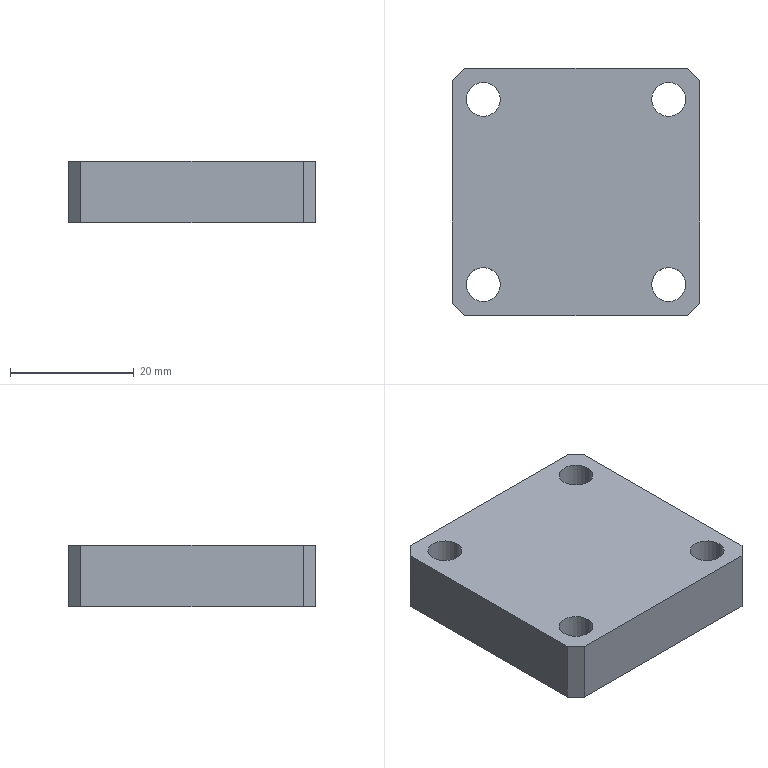Part | SolidWorks | features BaseBody 1 | 1 solid | 30 faces | box 40 x 40 x 10 mm | volume 13952 mm3 | cylinder 16 | plane 14 | commonest cylinder face diameters 5.5 x8 9.5 x8
STEP:
#1=CARTESIAN_POINT('',(19.75,15.,5.4));
#2=VERTEX_POINT('',#1);
#3=CARTESIAN_POINT('',(10.25,15.,5.4));
#4=VERTEX_POINT('',#3);
#5=CARTESIAN_POINT('',(15.,15.,5.4));
#6=DIRECTION('',(0.,0.,-1.));
#7=DIRECTION('',(-1.,0.,0.));
#8=AXIS2_PLACEMENT_3D('',#5,#6,#7);
#9=CIRCLE('',#8,4.75);
#10=EDGE_CURVE('',#2,#4,#9,.T.);
#11=ORIENTED_EDGE('',*,*,#10,.F.);
#12=CARTESIAN_POINT('',(19.75,15.,0.));
#13=VERTEX_POINT('',#12);
#14=CARTESIAN_POINT('',(19.75,15.,0.));
#15=DIRECTION('',(0.,0.,-1.));
#16=VECTOR('',#15,1000.);
#17=LINE('',#14,#16);
#18=EDGE_CURVE('',#2,#13,#17,.T.);
#19=ORIENTED_EDGE('',*,*,#18,.T.);
#20=CARTESIAN_POINT('',(10.25,15.,0.));
#21=VERTEX_POINT('',#20);
#22=CARTESIAN_POINT('',(15.,15.,0.));
#23=DIRECTION('',(0.,0.,-1.));
#24=DIRECTION('',(-1.,0.,0.));
#25=AXIS2_PLACEMENT_3D('',#22,#23,#24);
#26=CIRCLE('',#25,4.75);
#27=EDGE_CURVE('',#13,#21,#26,.T.);
#28=ORIENTED_EDGE('',*,*,#27,.T.);
#29=CARTESIAN_POINT('',(10.25,15.,0.));
#30=DIRECTION('',(0.,0.,-1.));
#31=VECTOR('',#30,1000.);
#32=LINE('',#29,#31);
#33=EDGE_CURVE('',#4,#21,#32,.T.);
#34=ORIENTED_EDGE('',*,*,#33,.F.);
#35=EDGE_LOOP('',(#11,#19,#28,#34));
#36=FACE_OUTER_BOUND('',#35,.T.);
#37=CARTESIAN_POINT('',(15.,15.,0.));
#38=DIRECTION('',(0.,0.,-1.));
#39=DIRECTION('',(-1.,0.,0.));
#40=AXIS2_PLACEMENT_3D('',#37,#38,#39);
#41=CYLINDRICAL_SURFACE('',#40,4.75);
#42=ADVANCED_FACE('',(#36),#41,.F.);
#43=CARTESIAN_POINT('',(17.75,15.,10.));
#44=VERTEX_POINT('',#43);
#45=CARTESIAN_POINT('',(12.25,15.,10.));
#46=VERTEX_POINT('',#45);
#47=CARTESIAN_POINT('',(15.,15.,10.));
#48=DIRECTION('',(0.,0.,-1.));
#49=DIRECTION('',(-1.,0.,0.));
#50=AXIS2_PLACEMENT_3D('',#47,#48,#49);
#51=CIRCLE('',#50,2.75);
#52=EDGE_CURVE('',#44,#46,#51,.T.);
#53=ORIENTED_EDGE('',*,*,#52,.F.);
#54=CARTESIAN_POINT('',(17.75,15.,5.4));
#55=VERTEX_POINT('',#54);
#56=CARTESIAN_POINT('',(17.75,15.,0.));
#57=DIRECTION('',(0.,0.,-1.));
#58=VECTOR('',#57,1000.);
#59=LINE('',#56,#58);
#60=EDGE_CURVE('',#44,#55,#59,.T.);
#61=ORIENTED_EDGE('',*,*,#60,.T.);
#62=CARTESIAN_POINT('',(12.25,15.,5.4));
#63=VERTEX_POINT('',#62);
#64=CARTESIAN_POINT('',(15.,15.,5.4));
#65=DIRECTION('',(0.,0.,-1.));
#66=DIRECTION('',(-1.,0.,0.));
#67=AXIS2_PLACEMENT_3D('',#64,#65,#66);
#68=CIRCLE('',#67,2.75);
#69=EDGE_CURVE('',#55,#63,#68,.T.);
#70=ORIENTED_EDGE('',*,*,#69,.T.);
#71=CARTESIAN_POINT('',(12.25,15.,0.));
#72=DIRECTION('',(0.,0.,-1.));
#73=VECTOR('',#72,1000.);
#74=LINE('',#71,#73);
#75=EDGE_CURVE('',#46,#63,#74,.T.);
#76=ORIENTED_EDGE('',*,*,#75,.F.);
#77=EDGE_LOOP('',(#53,#61,#70,#76));
#78=FACE_OUTER_BOUND('',#77,.T.);
#79=CARTESIAN_POINT('',(15.,15.,0.));
#80=DIRECTION('',(0.,0.,-1.));
#81=DIRECTION('',(-1.,0.,0.));
#82=AXIS2_PLACEMENT_3D('',#79,#80,#81);
#83=CYLINDRICAL_SURFACE('',#82,2.75);
#84=ADVANCED_FACE('',(#78),#83,.F.);
#85=CARTESIAN_POINT('',(-10.25,15.,5.4));
#86=VERTEX_POINT('',#85);
#87=CARTESIAN_POINT('',(-19.75,15.,5.4));
#88=VERTEX_POINT('',#87);
#89=CARTESIAN_POINT('',(-15.,15.,5.4));
#90=DIRECTION('',(0.,0.,-1.));
#91=DIRECTION('',(-1.,0.,0.));
#92=AXIS2_PLACEMENT_3D('',#89,#90,#91);
#93=CIRCLE('',#92,4.75);
#94=EDGE_CURVE('',#86,#88,#93,.T.);
#95=ORIENTED_EDGE('',*,*,#94,.F.);
#96=CARTESIAN_POINT('',(-10.25,15.,0.));
#97=VERTEX_POINT('',#96);
#98=CARTESIAN_POINT('',(-10.25,15.,0.));
#99=DIRECTION('',(0.,0.,-1.));
#100=VECTOR('',#99,1000.);
#101=LINE('',#98,#100);
#102=EDGE_CURVE('',#86,#97,#101,.T.);
#103=ORIENTED_EDGE('',*,*,#102,.T.);
#104=CARTESIAN_POINT('',(-19.75,15.,0.));
#105=VERTEX_POINT('',#104);
#106=CARTESIAN_POINT('',(-15.,15.,0.));
#107=DIRECTION('',(0.,0.,-1.));
#108=DIRECTION('',(-1.,0.,0.));
#109=AXIS2_PLACEMENT_3D('',#106,#107,#108);
#110=CIRCLE('',#109,4.75);
#111=EDGE_CURVE('',#97,#105,#110,.T.);
#112=ORIENTED_EDGE('',*,*,#111,.T.);
#113=CARTESIAN_POINT('',(-19.75,15.,0.));
#114=DIRECTION('',(0.,0.,-1.));
#115=VECTOR('',#114,1000.);
#116=LINE('',#113,#115);
#117=EDGE_CURVE('',#88,#105,#116,.T.);
#118=ORIENTED_EDGE('',*,*,#117,.F.);
#119=EDGE_LOOP('',(#95,#103,#112,#118));
#120=FACE_OUTER_BOUND('',#119,.T.);
#121=CARTESIAN_POINT('',(-15.,15.,0.));
#122=DIRECTION('',(0.,0.,-1.));
#123=DIRECTION('',(-1.,0.,0.));
#124=AXIS2_PLACEMENT_3D('',#121,#122,#123);
#125=CYLINDRICAL_SURFACE('',#124,4.75);
#126=ADVANCED_FACE('',(#120),#125,.F.);
#127=CARTESIAN_POINT('',(-12.25,15.,10.));
#128=VERTEX_POINT('',#127);
#129=CARTESIAN_POINT('',(-17.75,15.,10.));
#130=VERTEX_POINT('',#129);
#131=CARTESIAN_POINT('',(-15.,15.,10.));
#132=DIRECTION('',(0.,0.,-1.));
#133=DIRECTION('',(-1.,0.,0.));
#134=AXIS2_PLACEMENT_3D('',#131,#132,#133);
#135=CIRCLE('',#134,2.75);
#136=EDGE_CURVE('',#128,#130,#135,.T.);
#137=ORIENTED_EDGE('',*,*,#136,.F.);
#138=CARTESIAN_POINT('',(-12.25,15.,5.4));
#139=VERTEX_POINT('',#138);
#140=CARTESIAN_POINT('',(-12.25,15.,0.));
#141=DIRECTION('',(0.,0.,-1.));
#142=VECTOR('',#141,1000.);
#143=LINE('',#140,#142);
#144=EDGE_CURVE('',#128,#139,#143,.T.);
#145=ORIENTED_EDGE('',*,*,#144,.T.);
#146=CARTESIAN_POINT('',(-17.75,15.,5.4));
#147=VERTEX_POINT('',#146);
#148=CARTESIAN_POINT('',(-15.,15.,5.4));
#149=DIRECTION('',(0.,0.,-1.));
#150=DIRECTION('',(-1.,0.,0.));
#151=AXIS2_PLACEMENT_3D('',#148,#149,#150);
#152=CIRCLE('',#151,2.75);
#153=EDGE_CURVE('',#139,#147,#152,.T.);
#154=ORIENTED_EDGE('',*,*,#153,.T.);
#155=CARTESIAN_POINT('',(-17.75,15.,0.));
#156=DIRECTION('',(0.,0.,-1.));
#157=VECTOR('',#156,1000.);
#158=LINE('',#155,#157);
#159=EDGE_CURVE('',#130,#147,#158,.T.);
#160=ORIENTED_EDGE('',*,*,#159,.F.);
#161=EDGE_LOOP('',(#137,#145,#154,#160));
#162=FACE_OUTER_BOUND('',#161,.T.);
#163=CARTESIAN_POINT('',(-15.,15.,0.));
#164=DIRECTION('',(0.,0.,-1.));
#165=DIRECTION('',(-1.,0.,0.));
#166=AXIS2_PLACEMENT_3D('',#163,#164,#165);
#167=CYLINDRICAL_SURFACE('',#166,2.75);
#168=ADVANCED_FACE('',(#162),#167,.F.);
#169=CARTESIAN_POINT('',(19.75,-15.,5.4));
#170=VERTEX_POINT('',#169);
#171=CARTESIAN_POINT('',(10.25,-15.,5.4));
#172=VERTEX_POINT('',#171);
#173=CARTESIAN_POINT('',(15.,-15.,5.4));
#174=DIRECTION('',(0.,0.,-1.));
#175=DIRECTION('',(-1.,0.,0.));
#176=AXIS2_PLACEMENT_3D('',#173,#174,#175);
#177=CIRCLE('',#176,4.75);
#178=EDGE_CURVE('',#170,#172,#177,.T.);
#179=ORIENTED_EDGE('',*,*,#178,.F.);
#180=CARTESIAN_POINT('',(19.75,-15.,0.));
#181=VERTEX_POINT('',#180);
#182=CARTESIAN_POINT('',(19.75,-15.,0.));
#183=DIRECTION('',(0.,0.,-1.));
#184=VECTOR('',#183,1000.);
#185=LINE('',#182,#184);
#186=EDGE_CURVE('',#170,#181,#185,.T.);
#187=ORIENTED_EDGE('',*,*,#186,.T.);
#188=CARTESIAN_POINT('',(10.25,-15.,0.));
#189=VERTEX_POINT('',#188);
#190=CARTESIAN_POINT('',(15.,-15.,0.));
#191=DIRECTION('',(0.,0.,-1.));
#192=DIRECTION('',(-1.,0.,0.));
#193=AXIS2_PLACEMENT_3D('',#190,#191,#192);
#194=CIRCLE('',#193,4.75);
#195=EDGE_CURVE('',#181,#189,#194,.T.);
#196=ORIENTED_EDGE('',*,*,#195,.T.);
#197=CARTESIAN_POINT('',(10.25,-15.,0.));
#198=DIRECTION('',(0.,0.,-1.));
#199=VECTOR('',#198,1000.);
#200=LINE('',#197,#199);
#201=EDGE_CURVE('',#172,#189,#200,.T.);
#202=ORIENTED_EDGE('',*,*,#201,.F.);
#203=EDGE_LOOP('',(#179,#187,#196,#202));
#204=FACE_OUTER_BOUND('',#203,.T.);
#205=CARTESIAN_POINT('',(15.,-15.,0.));
#206=DIRECTION('',(0.,0.,-1.));
#207=DIRECTION('',(-1.,0.,0.));
#208=AXIS2_PLACEMENT_3D('',#205,#206,#207);
#209=CYLINDRICAL_SURFACE('',#208,4.75);
#210=ADVANCED_FACE('',(#204),#209,.F.);
#211=CARTESIAN_POINT('',(17.75,-15.,10.));
#212=VERTEX_POINT('',#211);
#213=CARTESIAN_POINT('',(12.25,-15.,10.));
#214=VERTEX_POINT('',#213);
#215=CARTESIAN_POINT('',(15.,-15.,10.));
#216=DIRECTION('',(0.,0.,-1.));
#217=DIRECTION('',(-1.,0.,0.));
#218=AXIS2_PLACEMENT_3D('',#215,#216,#217);
#219=CIRCLE('',#218,2.75);
#220=EDGE_CURVE('',#212,#214,#219,.T.);
#221=ORIENTED_EDGE('',*,*,#220,.F.);
#222=CARTESIAN_POINT('',(17.75,-15.,5.4));
#223=VERTEX_POINT('',#222);
#224=CARTESIAN_POINT('',(17.75,-15.,0.));
#225=DIRECTION('',(0.,0.,-1.));
#226=VECTOR('',#225,1000.);
#227=LINE('',#224,#226);
#228=EDGE_CURVE('',#212,#223,#227,.T.);
#229=ORIENTED_EDGE('',*,*,#228,.T.);
#230=CARTESIAN_POINT('',(12.25,-15.,5.4));
#231=VERTEX_POINT('',#230);
#232=CARTESIAN_POINT('',(15.,-15.,5.4));
#233=DIRECTION('',(0.,0.,-1.));
#234=DIRECTION('',(-1.,0.,0.));
#235=AXIS2_PLACEMENT_3D('',#232,#233,#234);
#236=CIRCLE('',#235,2.75);
#237=EDGE_CURVE('',#223,#231,#236,.T.);
#238=ORIENTED_EDGE('',*,*,#237,.T.);
#239=CARTESIAN_POINT('',(12.25,-15.,0.));
#240=DIRECTION('',(0.,0.,-1.));
#241=VECTOR('',#240,1000.);
#242=LINE('',#239,#241);
#243=EDGE_CURVE('',#214,#231,#242,.T.);
#244=ORIENTED_EDGE('',*,*,#243,.F.);
#245=EDGE_LOOP('',(#221,#229,#238,#244));
#246=FACE_OUTER_BOUND('',#245,.T.);
#247=CARTESIAN_POINT('',(15.,-15.,0.));
#248=DIRECTION('',(0.,0.,-1.));
#249=DIRECTION('',(-1.,0.,0.));
#250=AXIS2_PLACEMENT_3D('',#247,#248,#249);
#251=CYLINDRICAL_SURFACE('',#250,2.75);
#252=ADVANCED_FACE('',(#246),#251,.F.);
#253=CARTESIAN_POINT('',(-10.25,-15.,5.4));
#254=VERTEX_POINT('',#253);
#255=CARTESIAN_POINT('',(-19.75,-15.,5.4));
#256=VERTEX_POINT('',#255);
#257=CARTESIAN_POINT('',(-15.,-15.,5.4));
#258=DIRECTION('',(0.,0.,-1.));
#259=DIRECTION('',(-1.,0.,0.));
#260=AXIS2_PLACEMENT_3D('',#257,#258,#259);
#261=CIRCLE('',#260,4.75);
#262=EDGE_CURVE('',#254,#256,#261,.T.);
#263=ORIENTED_EDGE('',*,*,#262,.F.);
#264=CARTESIAN_POINT('',(-10.25,-15.,0.));
#265=VERTEX_POINT('',#264);
#266=CARTESIAN_POINT('',(-10.25,-15.,0.));
#267=DIRECTION('',(0.,0.,-1.));
#268=VECTOR('',#267,1000.);
#269=LINE('',#266,#268);
#270=EDGE_CURVE('',#254,#265,#269,.T.);
#271=ORIENTED_EDGE('',*,*,#270,.T.);
#272=CARTESIAN_POINT('',(-19.75,-15.,0.));
#273=VERTEX_POINT('',#272);
#274=CARTESIAN_POINT('',(-15.,-15.,0.));
#275=DIRECTION('',(0.,0.,-1.));
#276=DIRECTION('',(-1.,0.,0.));
#277=AXIS2_PLACEMENT_3D('',#274,#275,#276);
#278=CIRCLE('',#277,4.75);
#279=EDGE_CURVE('',#265,#273,#278,.T.);
#280=ORIENTED_EDGE('',*,*,#279,.T.);
#281=CARTESIAN_POINT('',(-19.75,-15.,0.));
#282=DIRECTION('',(0.,0.,-1.));
#283=VECTOR('',#282,1000.);
#284=LINE('',#281,#283);
#285=EDGE_CURVE('',#256,#273,#284,.T.);
#286=ORIENTED_EDGE('',*,*,#285,.F.);
#287=EDGE_LOOP('',(#263,#271,#280,#286));
#288=FACE_OUTER_BOUND('',#287,.T.);
#289=CARTESIAN_POINT('',(-15.,-15.,0.));
#290=DIRECTION('',(0.,0.,-1.));
#291=DIRECTION('',(-1.,0.,0.));
#292=AXIS2_PLACEMENT_3D('',#289,#290,#291);
#293=CYLINDRICAL_SURFACE('',#292,4.75);
#294=ADVANCED_FACE('',(#288),#293,.F.);
#295=CARTESIAN_POINT('',(-12.25,-15.,10.));
#296=VERTEX_POINT('',#295);
#297=CARTESIAN_POINT('',(-17.75,-15.,10.));
#298=VERTEX_POINT('',#297);
#299=CARTESIAN_POINT('',(-15.,-15.,10.));
#300=DIRECTION('',(0.,0.,-1.));
#301=DIRECTION('',(-1.,0.,0.));
#302=AXIS2_PLACEMENT_3D('',#299,#300,#301);
#303=CIRCLE('',#302,2.75);
#304=EDGE_CURVE('',#296,#298,#303,.T.);
#305=ORIENTED_EDGE('',*,*,#304,.F.);
#306=CARTESIAN_POINT('',(-12.25,-15.,5.4));
#307=VERTEX_POINT('',#306);
#308=CARTESIAN_POINT('',(-12.25,-15.,0.));
#309=DIRECTION('',(0.,0.,-1.));
#310=VECTOR('',#309,1000.);
#311=LINE('',#308,#310);
#312=EDGE_CURVE('',#296,#307,#311,.T.);
#313=ORIENTED_EDGE('',*,*,#312,.T.);
#314=CARTESIAN_POINT('',(-17.75,-15.,5.4));
#315=VERTEX_POINT('',#314);
#316=CARTESIAN_POINT('',(-15.,-15.,5.4));
#317=DIRECTION('',(0.,0.,-1.));
#318=DIRECTION('',(-1.,0.,0.));
#319=AXIS2_PLACEMENT_3D('',#316,#317,#318);
#320=CIRCLE('',#319,2.75);
#321=EDGE_CURVE('',#307,#315,#320,.T.);
#322=ORIENTED_EDGE('',*,*,#321,.T.);
#323=CARTESIAN_POINT('',(-17.75,-15.,0.));
#324=DIRECTION('',(0.,0.,-1.));
#325=VECTOR('',#324,1000.);
#326=LINE('',#323,#325);
#327=EDGE_CURVE('',#298,#315,#326,.T.);
#328=ORIENTED_EDGE('',*,*,#327,.F.);
#329=EDGE_LOOP('',(#305,#313,#322,#328));
#330=FACE_OUTER_BOUND('',#329,.T.);
#331=CARTESIAN_POINT('',(-15.,-15.,0.));
#332=DIRECTION('',(0.,0.,-1.));
#333=DIRECTION('',(-1.,0.,0.));
#334=AXIS2_PLACEMENT_3D('',#331,#332,#333);
#335=CYLINDRICAL_SURFACE('',#334,2.75);
#336=ADVANCED_FACE('',(#330),#335,.F.);
#337=CARTESIAN_POINT('',(-20.,18.,0.));
#338=VERTEX_POINT('',#337);
#339=CARTESIAN_POINT('',(-20.,-18.,0.));
#340=VERTEX_POINT('',#339);
#341=CARTESIAN_POINT('',(-20.,20.,0.));
#342=DIRECTION('',(0.,-1.,0.));
#343=VECTOR('',#342,1000.);
#344=LINE('',#341,#343);
#345=EDGE_CURVE('',#338,#340,#344,.T.);
#346=ORIENTED_EDGE('',*,*,#345,.T.);
#347=CARTESIAN_POINT('',(-20.,-18.,10.));
#348=VERTEX_POINT('',#347);
#349=CARTESIAN_POINT('',(-20.,-18.,10.));
#350=DIRECTION('',(0.,0.,1.));
#351=VECTOR('',#350,1000.);
#352=LINE('',#349,#351);
#353=EDGE_CURVE('',#340,#348,#352,.T.);
#354=ORIENTED_EDGE('',*,*,#353,.T.);
#355=CARTESIAN_POINT('',(-20.,18.,10.));
#356=VERTEX_POINT('',#355);
#357=CARTESIAN_POINT('',(-20.,20.,10.));
#358=DIRECTION('',(0.,-1.,0.));
#359=VECTOR('',#358,1000.);
#360=LINE('',#357,#359);
#361=EDGE_CURVE('',#356,#348,#360,.T.);
#362=ORIENTED_EDGE('',*,*,#361,.F.);
#363=CARTESIAN_POINT('',(-20.,18.,10.));
#364=DIRECTION('',(0.,0.,-1.));
#365=VECTOR('',#364,1000.);
#366=LINE('',#363,#365);
#367=EDGE_CURVE('',#356,#338,#366,.T.);
#368=ORIENTED_EDGE('',*,*,#367,.T.);
#369=EDGE_LOOP('',(#346,#354,#362,#368));
#370=FACE_OUTER_BOUND('',#369,.T.);
#371=CARTESIAN_POINT('',(-20.,20.,10.));
#372=DIRECTION('',(1.,0.,0.));
#373=DIRECTION('',(0.,1.,0.));
#374=AXIS2_PLACEMENT_3D('',#371,#372,#373);
#375=PLANE('',#374);
#376=ADVANCED_FACE('',(#370),#375,.F.);
#377=CARTESIAN_POINT('',(-18.,-20.,10.));
#378=VERTEX_POINT('',#377);
#379=CARTESIAN_POINT('',(18.,-20.,10.));
#380=VERTEX_POINT('',#379);
#381=CARTESIAN_POINT('',(20.,-20.,10.));
#382=DIRECTION('',(1.,0.,0.));
#383=VECTOR('',#382,1000.);
#384=LINE('',#381,#383);
#385=EDGE_CURVE('',#378,#380,#384,.T.);
#386=ORIENTED_EDGE('',*,*,#385,.F.);
#387=CARTESIAN_POINT('',(-18.,-20.,0.));
#388=VERTEX_POINT('',#387);
#389=CARTESIAN_POINT('',(-18.,-20.,10.));
#390=DIRECTION('',(0.,0.,-1.));
#391=VECTOR('',#390,1000.);
#392=LINE('',#389,#391);
#393=EDGE_CURVE('',#378,#388,#392,.T.);
#394=ORIENTED_EDGE('',*,*,#393,.T.);
#395=CARTESIAN_POINT('',(18.,-20.,0.));
#396=VERTEX_POINT('',#395);
#397=CARTESIAN_POINT('',(20.,-20.,0.));
#398=DIRECTION('',(1.,0.,0.));
#399=VECTOR('',#398,1000.);
#400=LINE('',#397,#399);
#401=EDGE_CURVE('',#388,#396,#400,.T.);
#402=ORIENTED_EDGE('',*,*,#401,.T.);
#403=CARTESIAN_POINT('',(18.,-20.,10.));
#404=DIRECTION('',(0.,0.,1.));
#405=VECTOR('',#404,1000.);
#406=LINE('',#403,#405);
#407=EDGE_CURVE('',#396,#380,#406,.T.);
#408=ORIENTED_EDGE('',*,*,#407,.T.);
#409=EDGE_LOOP('',(#386,#394,#402,#408));
#410=FACE_OUTER_BOUND('',#409,.T.);
#411=CARTESIAN_POINT('',(20.,-20.,10.));
#412=DIRECTION('',(0.,1.,0.));
#413=DIRECTION('',(-1.,0.,0.));
#414=AXIS2_PLACEMENT_3D('',#411,#412,#413);
#415=PLANE('',#414);
#416=ADVANCED_FACE('',(#410),#415,.F.);
#417=CARTESIAN_POINT('',(20.,-18.,10.));
#418=VERTEX_POINT('',#417);
#419=CARTESIAN_POINT('',(20.,18.,10.));
#420=VERTEX_POINT('',#419);
#421=CARTESIAN_POINT('',(20.,20.,10.));
#422=DIRECTION('',(0.,1.,0.));
#423=VECTOR('',#422,1000.);
#424=LINE('',#421,#423);
#425=EDGE_CURVE('',#418,#420,#424,.T.);
#426=ORIENTED_EDGE('',*,*,#425,.F.);
#427=CARTESIAN_POINT('',(20.,-18.,0.));
#428=VERTEX_POINT('',#427);
#429=CARTESIAN_POINT('',(20.,-18.,10.));
#430=DIRECTION('',(0.,0.,-1.));
#431=VECTOR('',#430,1000.);
#432=LINE('',#429,#431);
#433=EDGE_CURVE('',#418,#428,#432,.T.);
#434=ORIENTED_EDGE('',*,*,#433,.T.);
#435=CARTESIAN_POINT('',(20.,18.,0.));
#436=VERTEX_POINT('',#435);
#437=CARTESIAN_POINT('',(20.,20.,0.));
#438=DIRECTION('',(0.,1.,0.));
#439=VECTOR('',#438,1000.);
#440=LINE('',#437,#439);
#441=EDGE_CURVE('',#428,#436,#440,.T.);
#442=ORIENTED_EDGE('',*,*,#441,.T.);
#443=CARTESIAN_POINT('',(20.,18.,10.));
#444=DIRECTION('',(0.,0.,1.));
#445=VECTOR('',#444,1000.);
#446=LINE('',#443,#445);
#447=EDGE_CURVE('',#436,#420,#446,.T.);
#448=ORIENTED_EDGE('',*,*,#447,.T.);
#449=EDGE_LOOP('',(#426,#434,#442,#448));
#450=FACE_OUTER_BOUND('',#449,.T.);
#451=CARTESIAN_POINT('',(20.,20.,10.));
#452=DIRECTION('',(-1.,0.,0.));
#453=DIRECTION('',(0.,-1.,0.));
#454=AXIS2_PLACEMENT_3D('',#451,#452,#453);
#455=PLANE('',#454);
#456=ADVANCED_FACE('',(#450),#455,.F.);
#457=CARTESIAN_POINT('',(18.,20.,0.));
#458=VERTEX_POINT('',#457);
#459=CARTESIAN_POINT('',(-18.,20.,0.));
#460=VERTEX_POINT('',#459);
#461=CARTESIAN_POINT('',(20.,20.,0.));
#462=DIRECTION('',(-1.,0.,0.));
#463=VECTOR('',#462,1000.);
#464=LINE('',#461,#463);
#465=EDGE_CURVE('',#458,#460,#464,.T.);
#466=ORIENTED_EDGE('',*,*,#465,.T.);
#467=CARTESIAN_POINT('',(-18.,20.,10.));
#468=VERTEX_POINT('',#467);
#469=CARTESIAN_POINT('',(-18.,20.,10.));
#470=DIRECTION('',(0.,0.,1.));
#471=VECTOR('',#470,1000.);
#472=LINE('',#469,#471);
#473=EDGE_CURVE('',#460,#468,#472,.T.);
#474=ORIENTED_EDGE('',*,*,#473,.T.);
#475=CARTESIAN_POINT('',(18.,20.,10.));
#476=VERTEX_POINT('',#475);
#477=CARTESIAN_POINT('',(20.,20.,10.));
#478=DIRECTION('',(-1.,0.,0.));
#479=VECTOR('',#478,1000.);
#480=LINE('',#477,#479);
#481=EDGE_CURVE('',#476,#468,#480,.T.);
#482=ORIENTED_EDGE('',*,*,#481,.F.);
#483=CARTESIAN_POINT('',(18.,20.,10.));
#484=DIRECTION('',(0.,0.,-1.));
#485=VECTOR('',#484,1000.);
#486=LINE('',#483,#485);
#487=EDGE_CURVE('',#476,#458,#486,.T.);
#488=ORIENTED_EDGE('',*,*,#487,.T.);
#489=EDGE_LOOP('',(#466,#474,#482,#488));
#490=FACE_OUTER_BOUND('',#489,.T.);
#491=CARTESIAN_POINT('',(20.,20.,10.));
#492=DIRECTION('',(0.,-1.,0.));
#493=DIRECTION('',(1.,0.,0.));
#494=AXIS2_PLACEMENT_3D('',#491,#492,#493);
#495=PLANE('',#494);
#496=ADVANCED_FACE('',(#490),#495,.F.);
#497=CARTESIAN_POINT('',(15.,15.,10.));
#498=DIRECTION('',(0.,0.,-1.));
#499=DIRECTION('',(-1.,0.,0.));
#500=AXIS2_PLACEMENT_3D('',#497,#498,#499);
#501=CIRCLE('',#500,2.75);
#502=EDGE_CURVE('',#46,#44,#501,.T.);
#503=ORIENTED_EDGE('',*,*,#502,.T.);
#504=ORIENTED_EDGE('',*,*,#52,.T.);
#505=EDGE_LOOP('',(#503,#504));
#506=FACE_BOUND('',#505,.T.);
#507=CARTESIAN_POINT('',(-15.,15.,10.));
#508=DIRECTION('',(0.,0.,-1.));
#509=DIRECTION('',(-1.,0.,0.));
#510=AXIS2_PLACEMENT_3D('',#507,#508,#509);
#511=CIRCLE('',#510,2.75);
#512=EDGE_CURVE('',#130,#128,#511,.T.);
#513=ORIENTED_EDGE('',*,*,#512,.T.);
#514=ORIENTED_EDGE('',*,*,#136,.T.);
#515=EDGE_LOOP('',(#513,#514));
#516=FACE_BOUND('',#515,.T.);
#517=CARTESIAN_POINT('',(15.,-15.,10.));
#518=DIRECTION('',(0.,0.,-1.));
#519=DIRECTION('',(-1.,0.,0.));
#520=AXIS2_PLACEMENT_3D('',#517,#518,#519);
#521=CIRCLE('',#520,2.75);
#522=EDGE_CURVE('',#214,#212,#521,.T.);
#523=ORIENTED_EDGE('',*,*,#522,.T.);
#524=ORIENTED_EDGE('',*,*,#220,.T.);
#525=EDGE_LOOP('',(#523,#524));
#526=FACE_BOUND('',#525,.T.);
#527=CARTESIAN_POINT('',(-15.,-15.,10.));
#528=DIRECTION('',(0.,0.,-1.));
#529=DIRECTION('',(-1.,0.,0.));
#530=AXIS2_PLACEMENT_3D('',#527,#528,#529);
#531=CIRCLE('',#530,2.75);
#532=EDGE_CURVE('',#298,#296,#531,.T.);
#533=ORIENTED_EDGE('',*,*,#532,.T.);
#534=ORIENTED_EDGE('',*,*,#304,.T.);
#535=EDGE_LOOP('',(#533,#534));
#536=FACE_BOUND('',#535,.T.);
#537=ORIENTED_EDGE('',*,*,#361,.T.);
#538=CARTESIAN_POINT('',(-18.,-20.,10.));
#539=DIRECTION('',(0.7071,-0.7071,0.));
#540=VECTOR('',#539,1000.);
#541=LINE('',#538,#540);
#542=EDGE_CURVE('',#348,#378,#541,.T.);
#543=ORIENTED_EDGE('',*,*,#542,.T.);
#544=ORIENTED_EDGE('',*,*,#385,.T.);
#545=CARTESIAN_POINT('',(20.,-18.,10.));
#546=DIRECTION('',(0.7071,0.7071,0.));
#547=VECTOR('',#546,1000.);
#548=LINE('',#545,#547);
#549=EDGE_CURVE('',#380,#418,#548,.T.);
#550=ORIENTED_EDGE('',*,*,#549,.T.);
#551=ORIENTED_EDGE('',*,*,#425,.T.);
#552=CARTESIAN_POINT('',(18.,20.,10.));
#553=DIRECTION('',(-0.7071,0.7071,0.));
#554=VECTOR('',#553,1000.);
#555=LINE('',#552,#554);
#556=EDGE_CURVE('',#420,#476,#555,.T.);
#557=ORIENTED_EDGE('',*,*,#556,.T.);
#558=ORIENTED_EDGE('',*,*,#481,.T.);
#559=CARTESIAN_POINT('',(-20.,18.,10.));
#560=DIRECTION('',(-0.7071,-0.7071,0.));
#561=VECTOR('',#560,1000.);
#562=LINE('',#559,#561);
#563=EDGE_CURVE('',#468,#356,#562,.T.);
#564=ORIENTED_EDGE('',*,*,#563,.T.);
#565=EDGE_LOOP('',(#537,#543,#544,#550,#551,#557,#558,#564));
#566=FACE_OUTER_BOUND('',#565,.T.);
#567=CARTESIAN_POINT('',(0.,0.,10.));
#568=DIRECTION('',(0.,0.,-1.));
#569=DIRECTION('',(-1.,0.,0.));
#570=AXIS2_PLACEMENT_3D('',#567,#568,#569);
#571=PLANE('',#570);
#572=ADVANCED_FACE('',(#506,#516,#526,#536,#566),#571,.F.);
#573=CARTESIAN_POINT('',(15.,15.,0.));
#574=DIRECTION('',(0.,0.,-1.));
#575=DIRECTION('',(-1.,0.,0.));
#576=AXIS2_PLACEMENT_3D('',#573,#574,#575);
#577=CIRCLE('',#576,4.75);
#578=EDGE_CURVE('',#21,#13,#577,.T.);
#579=ORIENTED_EDGE('',*,*,#578,.F.);
#580=ORIENTED_EDGE('',*,*,#27,.F.);
#581=EDGE_LOOP('',(#579,#580));
#582=FACE_BOUND('',#581,.T.);
#583=CARTESIAN_POINT('',(-15.,15.,0.));
#584=DIRECTION('',(0.,0.,-1.));
#585=DIRECTION('',(-1.,0.,0.));
#586=AXIS2_PLACEMENT_3D('',#583,#584,#585);
#587=CIRCLE('',#586,4.75);
#588=EDGE_CURVE('',#105,#97,#587,.T.);
#589=ORIENTED_EDGE('',*,*,#588,.F.);
#590=ORIENTED_EDGE('',*,*,#111,.F.);
#591=EDGE_LOOP('',(#589,#590));
#592=FACE_BOUND('',#591,.T.);
#593=CARTESIAN_POINT('',(15.,-15.,0.));
#594=DIRECTION('',(0.,0.,-1.));
#595=DIRECTION('',(-1.,0.,0.));
#596=AXIS2_PLACEMENT_3D('',#593,#594,#595);
#597=CIRCLE('',#596,4.75);
#598=EDGE_CURVE('',#189,#181,#597,.T.);
#599=ORIENTED_EDGE('',*,*,#598,.F.);
#600=ORIENTED_EDGE('',*,*,#195,.F.);
#601=EDGE_LOOP('',(#599,#600));
#602=FACE_BOUND('',#601,.T.);
#603=CARTESIAN_POINT('',(-15.,-15.,0.));
#604=DIRECTION('',(0.,0.,-1.));
#605=DIRECTION('',(-1.,0.,0.));
#606=AXIS2_PLACEMENT_3D('',#603,#604,#605);
#607=CIRCLE('',#606,4.75);
#608=EDGE_CURVE('',#273,#265,#607,.T.);
#609=ORIENTED_EDGE('',*,*,#608,.F.);
#610=ORIENTED_EDGE('',*,*,#279,.F.);
#611=EDGE_LOOP('',(#609,#610));
#612=FACE_BOUND('',#611,.T.);
#613=ORIENTED_EDGE('',*,*,#401,.F.);
#614=CARTESIAN_POINT('',(-19.,-19.,0.));
#615=DIRECTION('',(-0.7071,0.7071,0.));
#616=VECTOR('',#615,1000.);
#617=LINE('',#614,#616);
#618=EDGE_CURVE('',#388,#340,#617,.T.);
#619=ORIENTED_EDGE('',*,*,#618,.T.);
#620=ORIENTED_EDGE('',*,*,#345,.F.);
#621=CARTESIAN_POINT('',(-19.,19.,0.));
#622=DIRECTION('',(0.7071,0.7071,0.));
#623=VECTOR('',#622,1000.);
#624=LINE('',#621,#623);
#625=EDGE_CURVE('',#338,#460,#624,.T.);
#626=ORIENTED_EDGE('',*,*,#625,.T.);
#627=ORIENTED_EDGE('',*,*,#465,.F.);
#628=CARTESIAN_POINT('',(19.,19.,0.));
#629=DIRECTION('',(0.7071,-0.7071,0.));
#630=VECTOR('',#629,1000.);
#631=LINE('',#628,#630);
#632=EDGE_CURVE('',#458,#436,#631,.T.);
#633=ORIENTED_EDGE('',*,*,#632,.T.);
#634=ORIENTED_EDGE('',*,*,#441,.F.);
#635=CARTESIAN_POINT('',(19.,-19.,0.));
#636=DIRECTION('',(-0.7071,-0.7071,0.));
#637=VECTOR('',#636,1000.);
#638=LINE('',#635,#637);
#639=EDGE_CURVE('',#428,#396,#638,.T.);
#640=ORIENTED_EDGE('',*,*,#639,.T.);
#641=EDGE_LOOP('',(#613,#619,#620,#626,#627,#633,#634,#640));
#642=FACE_OUTER_BOUND('',#641,.T.);
#643=CARTESIAN_POINT('',(0.,0.,0.));
#644=DIRECTION('',(0.,0.,-1.));
#645=DIRECTION('',(-1.,0.,0.));
#646=AXIS2_PLACEMENT_3D('',#643,#644,#645);
#647=PLANE('',#646);
#648=ADVANCED_FACE('',(#582,#592,#602,#612,#642),#647,.T.);
#649=ORIENTED_EDGE('',*,*,#312,.F.);
#650=ORIENTED_EDGE('',*,*,#532,.F.);
#651=ORIENTED_EDGE('',*,*,#327,.T.);
#652=CARTESIAN_POINT('',(-15.,-15.,5.4));
#653=DIRECTION('',(0.,0.,-1.));
#654=DIRECTION('',(-1.,0.,0.));
#655=AXIS2_PLACEMENT_3D('',#652,#653,#654);
#656=CIRCLE('',#655,2.75);
#657=EDGE_CURVE('',#315,#307,#656,.T.);
#658=ORIENTED_EDGE('',*,*,#657,.T.);
#659=EDGE_LOOP('',(#649,#650,#651,#658));
#660=FACE_OUTER_BOUND('',#659,.T.);
#661=CARTESIAN_POINT('',(-15.,-15.,0.));
#662=DIRECTION('',(0.,0.,-1.));
#663=DIRECTION('',(-1.,0.,0.));
#664=AXIS2_PLACEMENT_3D('',#661,#662,#663);
#665=CYLINDRICAL_SURFACE('',#664,2.75);
#666=ADVANCED_FACE('',(#660),#665,.F.);
#667=ORIENTED_EDGE('',*,*,#657,.F.);
#668=ORIENTED_EDGE('',*,*,#321,.F.);
#669=EDGE_LOOP('',(#667,#668));
#670=FACE_BOUND('',#669,.T.);
#671=CARTESIAN_POINT('',(-15.,-15.,5.4));
#672=DIRECTION('',(0.,0.,-1.));
#673=DIRECTION('',(-1.,0.,0.));
#674=AXIS2_PLACEMENT_3D('',#671,#672,#673);
#675=CIRCLE('',#674,4.75);
#676=EDGE_CURVE('',#256,#254,#675,.T.);
#677=ORIENTED_EDGE('',*,*,#676,.T.);
#678=ORIENTED_EDGE('',*,*,#262,.T.);
#679=EDGE_LOOP('',(#677,#678));
#680=FACE_OUTER_BOUND('',#679,.T.);
#681=CARTESIAN_POINT('',(-12.25,-15.,5.4));
#682=DIRECTION('',(0.,0.,1.));
#683=DIRECTION('',(1.,0.,0.));
#684=AXIS2_PLACEMENT_3D('',#681,#682,#683);
#685=PLANE('',#684);
#686=ADVANCED_FACE('',(#670,#680),#685,.F.);
#687=ORIENTED_EDGE('',*,*,#270,.F.);
#688=ORIENTED_EDGE('',*,*,#676,.F.);
#689=ORIENTED_EDGE('',*,*,#285,.T.);
#690=ORIENTED_EDGE('',*,*,#608,.T.);
#691=EDGE_LOOP('',(#687,#688,#689,#690));
#692=FACE_OUTER_BOUND('',#691,.T.);
#693=CARTESIAN_POINT('',(-15.,-15.,0.));
#694=DIRECTION('',(0.,0.,-1.));
#695=DIRECTION('',(-1.,0.,0.));
#696=AXIS2_PLACEMENT_3D('',#693,#694,#695);
#697=CYLINDRICAL_SURFACE('',#696,4.75);
#698=ADVANCED_FACE('',(#692),#697,.F.);
#699=ORIENTED_EDGE('',*,*,#228,.F.);
#700=ORIENTED_EDGE('',*,*,#522,.F.);
#701=ORIENTED_EDGE('',*,*,#243,.T.);
#702=CARTESIAN_POINT('',(15.,-15.,5.4));
#703=DIRECTION('',(0.,0.,-1.));
#704=DIRECTION('',(-1.,0.,0.));
#705=AXIS2_PLACEMENT_3D('',#702,#703,#704);
#706=CIRCLE('',#705,2.75);
#707=EDGE_CURVE('',#231,#223,#706,.T.);
#708=ORIENTED_EDGE('',*,*,#707,.T.);
#709=EDGE_LOOP('',(#699,#700,#701,#708));
#710=FACE_OUTER_BOUND('',#709,.T.);
#711=CARTESIAN_POINT('',(15.,-15.,0.));
#712=DIRECTION('',(0.,0.,-1.));
#713=DIRECTION('',(-1.,0.,0.));
#714=AXIS2_PLACEMENT_3D('',#711,#712,#713);
#715=CYLINDRICAL_SURFACE('',#714,2.75);
#716=ADVANCED_FACE('',(#710),#715,.F.);
#717=ORIENTED_EDGE('',*,*,#707,.F.);
#718=ORIENTED_EDGE('',*,*,#237,.F.);
#719=EDGE_LOOP('',(#717,#718));
#720=FACE_BOUND('',#719,.T.);
#721=CARTESIAN_POINT('',(15.,-15.,5.4));
#722=DIRECTION('',(0.,0.,-1.));
#723=DIRECTION('',(-1.,0.,0.));
#724=AXIS2_PLACEMENT_3D('',#721,#722,#723);
#725=CIRCLE('',#724,4.75);
#726=EDGE_CURVE('',#172,#170,#725,.T.);
#727=ORIENTED_EDGE('',*,*,#726,.T.);
#728=ORIENTED_EDGE('',*,*,#178,.T.);
#729=EDGE_LOOP('',(#727,#728));
#730=FACE_OUTER_BOUND('',#729,.T.);
#731=CARTESIAN_POINT('',(17.75,-15.,5.4));
#732=DIRECTION('',(0.,0.,1.));
#733=DIRECTION('',(1.,0.,0.));
#734=AXIS2_PLACEMENT_3D('',#731,#732,#733);
#735=PLANE('',#734);
#736=ADVANCED_FACE('',(#720,#730),#735,.F.);
#737=ORIENTED_EDGE('',*,*,#186,.F.);
#738=ORIENTED_EDGE('',*,*,#726,.F.);
#739=ORIENTED_EDGE('',*,*,#201,.T.);
#740=ORIENTED_EDGE('',*,*,#598,.T.);
#741=EDGE_LOOP('',(#737,#738,#739,#740));
#742=FACE_OUTER_BOUND('',#741,.T.);
#743=CARTESIAN_POINT('',(15.,-15.,0.));
#744=DIRECTION('',(0.,0.,-1.));
#745=DIRECTION('',(-1.,0.,0.));
#746=AXIS2_PLACEMENT_3D('',#743,#744,#745);
#747=CYLINDRICAL_SURFACE('',#746,4.75);
#748=ADVANCED_FACE('',(#742),#747,.F.);
#749=ORIENTED_EDGE('',*,*,#144,.F.);
#750=ORIENTED_EDGE('',*,*,#512,.F.);
#751=ORIENTED_EDGE('',*,*,#159,.T.);
#752=CARTESIAN_POINT('',(-15.,15.,5.4));
#753=DIRECTION('',(0.,0.,-1.));
#754=DIRECTION('',(-1.,0.,0.));
#755=AXIS2_PLACEMENT_3D('',#752,#753,#754);
#756=CIRCLE('',#755,2.75);
#757=EDGE_CURVE('',#147,#139,#756,.T.);
#758=ORIENTED_EDGE('',*,*,#757,.T.);
#759=EDGE_LOOP('',(#749,#750,#751,#758));
#760=FACE_OUTER_BOUND('',#759,.T.);
#761=CARTESIAN_POINT('',(-15.,15.,0.));
#762=DIRECTION('',(0.,0.,-1.));
#763=DIRECTION('',(-1.,0.,0.));
#764=AXIS2_PLACEMENT_3D('',#761,#762,#763);
#765=CYLINDRICAL_SURFACE('',#764,2.75);
#766=ADVANCED_FACE('',(#760),#765,.F.);
#767=ORIENTED_EDGE('',*,*,#757,.F.);
#768=ORIENTED_EDGE('',*,*,#153,.F.);
#769=EDGE_LOOP('',(#767,#768));
#770=FACE_BOUND('',#769,.T.);
#771=CARTESIAN_POINT('',(-15.,15.,5.4));
#772=DIRECTION('',(0.,0.,-1.));
#773=DIRECTION('',(-1.,0.,0.));
#774=AXIS2_PLACEMENT_3D('',#771,#772,#773);
#775=CIRCLE('',#774,4.75);
#776=EDGE_CURVE('',#88,#86,#775,.T.);
#777=ORIENTED_EDGE('',*,*,#776,.T.);
#778=ORIENTED_EDGE('',*,*,#94,.T.);
#779=EDGE_LOOP('',(#777,#778));
#780=FACE_OUTER_BOUND('',#779,.T.);
#781=CARTESIAN_POINT('',(-12.25,15.,5.4));
#782=DIRECTION('',(0.,0.,1.));
#783=DIRECTION('',(1.,0.,0.));
#784=AXIS2_PLACEMENT_3D('',#781,#782,#783);
#785=PLANE('',#784);
#786=ADVANCED_FACE('',(#770,#780),#785,.F.);
#787=ORIENTED_EDGE('',*,*,#102,.F.);
#788=ORIENTED_EDGE('',*,*,#776,.F.);
#789=ORIENTED_EDGE('',*,*,#117,.T.);
#790=ORIENTED_EDGE('',*,*,#588,.T.);
#791=EDGE_LOOP('',(#787,#788,#789,#790));
#792=FACE_OUTER_BOUND('',#791,.T.);
#793=CARTESIAN_POINT('',(-15.,15.,0.));
#794=DIRECTION('',(0.,0.,-1.));
#795=DIRECTION('',(-1.,0.,0.));
#796=AXIS2_PLACEMENT_3D('',#793,#794,#795);
#797=CYLINDRICAL_SURFACE('',#796,4.75);
#798=ADVANCED_FACE('',(#792),#797,.F.);
#799=ORIENTED_EDGE('',*,*,#60,.F.);
#800=ORIENTED_EDGE('',*,*,#502,.F.);
#801=ORIENTED_EDGE('',*,*,#75,.T.);
#802=CARTESIAN_POINT('',(15.,15.,5.4));
#803=DIRECTION('',(0.,0.,-1.));
#804=DIRECTION('',(-1.,0.,0.));
#805=AXIS2_PLACEMENT_3D('',#802,#803,#804);
#806=CIRCLE('',#805,2.75);
#807=EDGE_CURVE('',#63,#55,#806,.T.);
#808=ORIENTED_EDGE('',*,*,#807,.T.);
#809=EDGE_LOOP('',(#799,#800,#801,#808));
#810=FACE_OUTER_BOUND('',#809,.T.);
#811=CARTESIAN_POINT('',(15.,15.,0.));
#812=DIRECTION('',(0.,0.,-1.));
#813=DIRECTION('',(-1.,0.,0.));
#814=AXIS2_PLACEMENT_3D('',#811,#812,#813);
#815=CYLINDRICAL_SURFACE('',#814,2.75);
#816=ADVANCED_FACE('',(#810),#815,.F.);
#817=ORIENTED_EDGE('',*,*,#807,.F.);
#818=ORIENTED_EDGE('',*,*,#69,.F.);
#819=EDGE_LOOP('',(#817,#818));
#820=FACE_BOUND('',#819,.T.);
#821=CARTESIAN_POINT('',(15.,15.,5.4));
#822=DIRECTION('',(0.,0.,-1.));
#823=DIRECTION('',(-1.,0.,0.));
#824=AXIS2_PLACEMENT_3D('',#821,#822,#823);
#825=CIRCLE('',#824,4.75);
#826=EDGE_CURVE('',#4,#2,#825,.T.);
#827=ORIENTED_EDGE('',*,*,#826,.T.);
#828=ORIENTED_EDGE('',*,*,#10,.T.);
#829=EDGE_LOOP('',(#827,#828));
#830=FACE_OUTER_BOUND('',#829,.T.);
#831=CARTESIAN_POINT('',(17.75,15.,5.4));
#832=DIRECTION('',(0.,0.,1.));
#833=DIRECTION('',(1.,0.,0.));
#834=AXIS2_PLACEMENT_3D('',#831,#832,#833);
#835=PLANE('',#834);
#836=ADVANCED_FACE('',(#820,#830),#835,.F.);
#837=ORIENTED_EDGE('',*,*,#18,.F.);
#838=ORIENTED_EDGE('',*,*,#826,.F.);
#839=ORIENTED_EDGE('',*,*,#33,.T.);
#840=ORIENTED_EDGE('',*,*,#578,.T.);
#841=EDGE_LOOP('',(#837,#838,#839,#840));
#842=FACE_OUTER_BOUND('',#841,.T.);
#843=CARTESIAN_POINT('',(15.,15.,0.));
#844=DIRECTION('',(0.,0.,-1.));
#845=DIRECTION('',(-1.,0.,0.));
#846=AXIS2_PLACEMENT_3D('',#843,#844,#845);
#847=CYLINDRICAL_SURFACE('',#846,4.75);
#848=ADVANCED_FACE('',(#842),#847,.F.);
#849=ORIENTED_EDGE('',*,*,#542,.F.);
#850=ORIENTED_EDGE('',*,*,#353,.F.);
#851=ORIENTED_EDGE('',*,*,#618,.F.);
#852=ORIENTED_EDGE('',*,*,#393,.F.);
#853=EDGE_LOOP('',(#849,#850,#851,#852));
#854=FACE_OUTER_BOUND('',#853,.T.);
#855=CARTESIAN_POINT('',(-18.,-20.,10.));
#856=DIRECTION('',(0.7071,0.7071,0.));
#857=DIRECTION('',(0.,0.,-1.));
#858=AXIS2_PLACEMENT_3D('',#855,#856,#857);
#859=PLANE('',#858);
#860=ADVANCED_FACE('',(#854),#859,.F.);
#861=ORIENTED_EDGE('',*,*,#549,.F.);
#862=ORIENTED_EDGE('',*,*,#407,.F.);
#863=ORIENTED_EDGE('',*,*,#639,.F.);
#864=ORIENTED_EDGE('',*,*,#433,.F.);
#865=EDGE_LOOP('',(#861,#862,#863,#864));
#866=FACE_OUTER_BOUND('',#865,.T.);
#867=CARTESIAN_POINT('',(20.,-18.,10.));
#868=DIRECTION('',(-0.7071,0.7071,0.));
#869=DIRECTION('',(0.,0.,-1.));
#870=AXIS2_PLACEMENT_3D('',#867,#868,#869);
#871=PLANE('',#870);
#872=ADVANCED_FACE('',(#866),#871,.F.);
#873=ORIENTED_EDGE('',*,*,#563,.F.);
#874=ORIENTED_EDGE('',*,*,#473,.F.);
#875=ORIENTED_EDGE('',*,*,#625,.F.);
#876=ORIENTED_EDGE('',*,*,#367,.F.);
#877=EDGE_LOOP('',(#873,#874,#875,#876));
#878=FACE_OUTER_BOUND('',#877,.T.);
#879=CARTESIAN_POINT('',(-20.,18.,10.));
#880=DIRECTION('',(0.7071,-0.7071,0.));
#881=DIRECTION('',(0.,0.,-1.));
#882=AXIS2_PLACEMENT_3D('',#879,#880,#881);
#883=PLANE('',#882);
#884=ADVANCED_FACE('',(#878),#883,.F.);
#885=ORIENTED_EDGE('',*,*,#556,.F.);
#886=ORIENTED_EDGE('',*,*,#447,.F.);
#887=ORIENTED_EDGE('',*,*,#632,.F.);
#888=ORIENTED_EDGE('',*,*,#487,.F.);
#889=EDGE_LOOP('',(#885,#886,#887,#888));
#890=FACE_OUTER_BOUND('',#889,.T.);
#891=CARTESIAN_POINT('',(18.,20.,10.));
#892=DIRECTION('',(-0.7071,-0.7071,0.));
#893=DIRECTION('',(0.,0.,-1.));
#894=AXIS2_PLACEMENT_3D('',#891,#892,#893);
#895=PLANE('',#894);
#896=ADVANCED_FACE('',(#890),#895,.F.);
#897=CLOSED_SHELL('',(#42,#84,#126,#168,#210,#252,#294,#336,#376,#416,#456,#496,#572,#648,#666,#686,#698,#716,#736,#748,#766,#786,#798,#816,#836,#848,#860,#872,#884,#896));
#898=MANIFOLD_SOLID_BREP('',#897);
#899=CARTESIAN_POINT('',(0.,0.,0.));
#900=DIRECTION('',(0.,0.,1.));
#901=DIRECTION('',(1.,0.,0.));
#902=AXIS2_PLACEMENT_3D('',#899,#900,#901);
#903=(LENGTH_UNIT()NAMED_UNIT(*)SI_UNIT(.MILLI.,.METRE.));
#904=UNCERTAINTY_MEASURE_WITH_UNIT(LENGTH_MEASURE(0.00001),#903,'','');
#905=(NAMED_UNIT(*)PLANE_ANGLE_UNIT()SI_UNIT($,.RADIAN.));
#906=(NAMED_UNIT(*)SI_UNIT($,.STERADIAN.)SOLID_ANGLE_UNIT());
#907=(GEOMETRIC_REPRESENTATION_CONTEXT(3)GLOBAL_UNCERTAINTY_ASSIGNED_CONTEXT((#904))GLOBAL_UNIT_ASSIGNED_CONTEXT((#903,#905,#906))REPRESENTATION_CONTEXT('',''));
#908=ADVANCED_BREP_SHAPE_REPRESENTATION('',(#898,#902),#907);